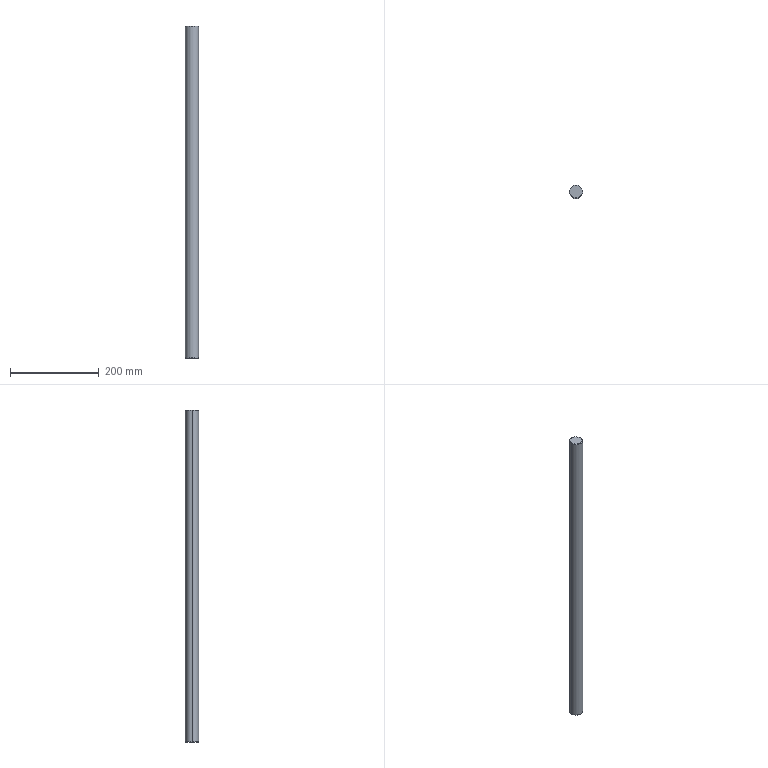Part | STEP file | 2003 Bag feed support shaft | 1 solid | 12 faces | box 30 x 30 x 750 mm | volume 528443 mm3 | cone 6 | cylinder 4 | plane 2 | commonest cylinder face diameters 8.5 x2 30 x2
STEP:
#1=CARTESIAN_POINT('',(0.,0.,0.));
#2=DIRECTION('',(0.,0.,1.));
#3=DIRECTION('',(1.,0.,0.));
#4=AXIS2_PLACEMENT_3D('',#1,#2,#3);
#5=CARTESIAN_POINT('',(-14.,0.,0.));
#6=VERTEX_POINT('',#5);
#7=CARTESIAN_POINT('',(14.,0.,0.));
#8=VERTEX_POINT('',#7);
#9=CARTESIAN_POINT('',(0.,0.,0.));
#10=DIRECTION('',(0.,0.,-1.));
#11=DIRECTION('',(1.,0.,0.));
#12=AXIS2_PLACEMENT_3D('',#9,#10,#11);
#13=CIRCLE('',#12,14.);
#14=CARTESIAN_POINT('',(0.,0.,1.));
#15=DIRECTION('',(0.,0.,1.));
#16=DIRECTION('',(1.,0.,0.));
#17=AXIS2_PLACEMENT_3D('',#14,#15,#16);
#18=CONICAL_SURFACE('',#17,15.,0.7854);
#19=CARTESIAN_POINT('',(6.283,-1.));
#20=DIRECTION('',(-1.,0.));
#21=VECTOR('',#20,1.);
#22=LINE('',#19,#21);
#23=(GEOMETRIC_REPRESENTATION_CONTEXT(2)PARAMETRIC_REPRESENTATION_CONTEXT()REPRESENTATION_CONTEXT('',''));
#24=DEFINITIONAL_REPRESENTATION('',(#22),#23);
#25=PCURVE('',#18,#24);
#26=CARTESIAN_POINT('',(0.,0.,0.));
#27=DIRECTION('',(0.,0.,1.));
#28=DIRECTION('',(1.,0.,0.));
#29=AXIS2_PLACEMENT_3D('',#26,#27,#28);
#30=PLANE('',#29);
#31=CARTESIAN_POINT('',(14.,0.));
#32=CARTESIAN_POINT('',(14.,-24.249));
#33=CARTESIAN_POINT('',(-7.,-12.124));
#34=CARTESIAN_POINT('',(-28.,0.));
#35=CARTESIAN_POINT('',(-7.,12.124));
#36=CARTESIAN_POINT('',(14.,24.249));
#37=CARTESIAN_POINT('',(14.,0.));
#38=(BOUNDED_CURVE()B_SPLINE_CURVE(2,(#31,#32,#33,#34,#35,#36,#37),.UNSPECIFIED.,.T.,.F.)B_SPLINE_CURVE_WITH_KNOTS((1,2,2,2,2,1),(-2.094,0.,2.094,4.189,6.283,8.378),.UNSPECIFIED.)CURVE()GEOMETRIC_REPRESENTATION_ITEM()RATIONAL_B_SPLINE_CURVE((1.,0.5,1.,0.5,1.,0.5,1.))REPRESENTATION_ITEM(''));
#39=(GEOMETRIC_REPRESENTATION_CONTEXT(2)PARAMETRIC_REPRESENTATION_CONTEXT()REPRESENTATION_CONTEXT('',''));
#40=DEFINITIONAL_REPRESENTATION('',(#38),#39);
#41=PCURVE('',#30,#40);
#42=SURFACE_CURVE('',#13,(#25,#41),.PCURVE_S1.);
#43=EDGE_CURVE('',#6,#8,#42,.T.);
#44=ORIENTED_EDGE('',*,*,#43,.F.);
#45=CARTESIAN_POINT('',(-15.,0.,1.));
#46=VERTEX_POINT('',#45);
#47=CARTESIAN_POINT('',(-15.,0.,1.));
#48=DIRECTION('',(-0.7071,0.,0.7071));
#49=VECTOR('',#48,1.);
#50=LINE('',#47,#49);
#51=CARTESIAN_POINT('',(3.142,0.));
#52=DIRECTION('',(0.,1.));
#53=VECTOR('',#52,1.);
#54=LINE('',#51,#53);
#55=(GEOMETRIC_REPRESENTATION_CONTEXT(2)PARAMETRIC_REPRESENTATION_CONTEXT()REPRESENTATION_CONTEXT('',''));
#56=DEFINITIONAL_REPRESENTATION('',(#54),#55);
#57=PCURVE('',#18,#56);
#58=CARTESIAN_POINT('',(0.,0.,1.));
#59=DIRECTION('',(0.,0.,1.));
#60=DIRECTION('',(1.,0.,0.));
#61=AXIS2_PLACEMENT_3D('',#58,#59,#60);
#62=CONICAL_SURFACE('',#61,15.,0.7854);
#63=CARTESIAN_POINT('',(3.142,0.));
#64=DIRECTION('',(0.,1.));
#65=VECTOR('',#64,1.);
#66=LINE('',#63,#65);
#67=(GEOMETRIC_REPRESENTATION_CONTEXT(2)PARAMETRIC_REPRESENTATION_CONTEXT()REPRESENTATION_CONTEXT('',''));
#68=DEFINITIONAL_REPRESENTATION('',(#66),#67);
#69=PCURVE('',#62,#68);
#70=SURFACE_CURVE('',#50,(#57,#69),.PCURVE_S1.);
#71=EDGE_CURVE('',#6,#46,#70,.T.);
#72=ORIENTED_EDGE('',*,*,#71,.T.);
#73=CARTESIAN_POINT('',(15.,0.,1.));
#74=VERTEX_POINT('',#73);
#75=CARTESIAN_POINT('',(0.,0.,1.));
#76=DIRECTION('',(0.,0.,1.));
#77=DIRECTION('',(1.,0.,0.));
#78=AXIS2_PLACEMENT_3D('',#75,#76,#77);
#79=CIRCLE('',#78,15.);
#80=CARTESIAN_POINT('',(0.,0.));
#81=DIRECTION('',(1.,0.));
#82=VECTOR('',#81,1.);
#83=LINE('',#80,#82);
#84=(GEOMETRIC_REPRESENTATION_CONTEXT(2)PARAMETRIC_REPRESENTATION_CONTEXT()REPRESENTATION_CONTEXT('',''));
#85=DEFINITIONAL_REPRESENTATION('',(#83),#84);
#86=PCURVE('',#18,#85);
#87=CARTESIAN_POINT('',(0.,0.,750.));
#88=DIRECTION('',(0.,0.,-1.));
#89=DIRECTION('',(-1.,0.,0.));
#90=AXIS2_PLACEMENT_3D('',#87,#88,#89);
#91=CYLINDRICAL_SURFACE('',#90,15.);
#92=CARTESIAN_POINT('',(3.142,749.));
#93=DIRECTION('',(-1.,0.));
#94=VECTOR('',#93,1.);
#95=LINE('',#92,#94);
#96=(GEOMETRIC_REPRESENTATION_CONTEXT(2)PARAMETRIC_REPRESENTATION_CONTEXT()REPRESENTATION_CONTEXT('',''));
#97=DEFINITIONAL_REPRESENTATION('',(#95),#96);
#98=PCURVE('',#91,#97);
#99=SURFACE_CURVE('',#79,(#86,#98),.PCURVE_S1.);
#100=EDGE_CURVE('',#74,#46,#99,.T.);
#101=ORIENTED_EDGE('',*,*,#100,.F.);
#102=CARTESIAN_POINT('',(15.,0.,1.));
#103=DIRECTION('',(0.7071,0.,0.7071));
#104=VECTOR('',#103,1.);
#105=LINE('',#102,#104);
#106=CARTESIAN_POINT('',(0.,0.));
#107=DIRECTION('',(0.,1.));
#108=VECTOR('',#107,1.);
#109=LINE('',#106,#108);
#110=(GEOMETRIC_REPRESENTATION_CONTEXT(2)PARAMETRIC_REPRESENTATION_CONTEXT()REPRESENTATION_CONTEXT('',''));
#111=DEFINITIONAL_REPRESENTATION('',(#109),#110);
#112=PCURVE('',#18,#111);
#113=CARTESIAN_POINT('',(6.283,0.));
#114=DIRECTION('',(0.,1.));
#115=VECTOR('',#114,1.);
#116=LINE('',#113,#115);
#117=(GEOMETRIC_REPRESENTATION_CONTEXT(2)PARAMETRIC_REPRESENTATION_CONTEXT()REPRESENTATION_CONTEXT('',''));
#118=DEFINITIONAL_REPRESENTATION('',(#116),#117);
#119=PCURVE('',#62,#118);
#120=SURFACE_CURVE('',#105,(#112,#119),.PCURVE_S1.);
#121=EDGE_CURVE('',#8,#74,#120,.T.);
#122=ORIENTED_EDGE('',*,*,#121,.F.);
#123=EDGE_LOOP('',(#44,#72,#101,#122));
#124=FACE_BOUND('',#123,.T.);
#125=ADVANCED_FACE('',(#124),#18,.T.);
#126=CARTESIAN_POINT('',(14.,0.,750.));
#127=VERTEX_POINT('',#126);
#128=CARTESIAN_POINT('',(-14.,0.,750.));
#129=VERTEX_POINT('',#128);
#130=CARTESIAN_POINT('',(0.,0.,750.));
#131=DIRECTION('',(0.,0.,1.));
#132=DIRECTION('',(1.,0.,0.));
#133=AXIS2_PLACEMENT_3D('',#130,#131,#132);
#134=CIRCLE('',#133,14.);
#135=CARTESIAN_POINT('',(0.,0.,750.));
#136=DIRECTION('',(0.,0.,-1.));
#137=DIRECTION('',(-1.,0.,0.));
#138=AXIS2_PLACEMENT_3D('',#135,#136,#137);
#139=CONICAL_SURFACE('',#138,14.,0.7854);
#140=CARTESIAN_POINT('',(3.142,0.));
#141=DIRECTION('',(-1.,0.));
#142=VECTOR('',#141,1.);
#143=LINE('',#140,#142);
#144=(GEOMETRIC_REPRESENTATION_CONTEXT(2)PARAMETRIC_REPRESENTATION_CONTEXT()REPRESENTATION_CONTEXT('',''));
#145=DEFINITIONAL_REPRESENTATION('',(#143),#144);
#146=PCURVE('',#139,#145);
#147=CARTESIAN_POINT('',(0.,0.,750.));
#148=DIRECTION('',(0.,0.,1.));
#149=DIRECTION('',(1.,0.,0.));
#150=AXIS2_PLACEMENT_3D('',#147,#148,#149);
#151=PLANE('',#150);
#152=CARTESIAN_POINT('',(0.,0.));
#153=DIRECTION('',(1.,0.));
#154=AXIS2_PLACEMENT_2D('',#152,#153);
#155=CIRCLE('',#154,14.);
#156=(GEOMETRIC_REPRESENTATION_CONTEXT(2)PARAMETRIC_REPRESENTATION_CONTEXT()REPRESENTATION_CONTEXT('',''));
#157=DEFINITIONAL_REPRESENTATION('',(#155),#156);
#158=PCURVE('',#151,#157);
#159=SURFACE_CURVE('',#134,(#146,#158),.PCURVE_S1.);
#160=EDGE_CURVE('',#127,#129,#159,.T.);
#161=ORIENTED_EDGE('',*,*,#160,.F.);
#162=CARTESIAN_POINT('',(15.,0.,749.));
#163=VERTEX_POINT('',#162);
#164=CARTESIAN_POINT('',(14.,0.,750.));
#165=DIRECTION('',(0.7071,0.,-0.7071));
#166=VECTOR('',#165,1.);
#167=LINE('',#164,#166);
#168=CARTESIAN_POINT('',(3.142,0.));
#169=DIRECTION('',(0.,1.));
#170=VECTOR('',#169,1.);
#171=LINE('',#168,#170);
#172=(GEOMETRIC_REPRESENTATION_CONTEXT(2)PARAMETRIC_REPRESENTATION_CONTEXT()REPRESENTATION_CONTEXT('',''));
#173=DEFINITIONAL_REPRESENTATION('',(#171),#172);
#174=PCURVE('',#139,#173);
#175=CARTESIAN_POINT('',(0.,0.,750.));
#176=DIRECTION('',(0.,0.,-1.));
#177=DIRECTION('',(-1.,0.,0.));
#178=AXIS2_PLACEMENT_3D('',#175,#176,#177);
#179=CONICAL_SURFACE('',#178,14.,0.7854);
#180=CARTESIAN_POINT('',(3.142,0.));
#181=DIRECTION('',(0.,1.));
#182=VECTOR('',#181,1.);
#183=LINE('',#180,#182);
#184=(GEOMETRIC_REPRESENTATION_CONTEXT(2)PARAMETRIC_REPRESENTATION_CONTEXT()REPRESENTATION_CONTEXT('',''));
#185=DEFINITIONAL_REPRESENTATION('',(#183),#184);
#186=PCURVE('',#179,#185);
#187=SURFACE_CURVE('',#167,(#174,#186),.PCURVE_S1.);
#188=EDGE_CURVE('',#127,#163,#187,.T.);
#189=ORIENTED_EDGE('',*,*,#188,.T.);
#190=CARTESIAN_POINT('',(-15.,0.,749.));
#191=VERTEX_POINT('',#190);
#192=CARTESIAN_POINT('',(0.,0.,749.));
#193=DIRECTION('',(0.,0.,-1.));
#194=DIRECTION('',(1.,0.,0.));
#195=AXIS2_PLACEMENT_3D('',#192,#193,#194);
#196=CIRCLE('',#195,15.);
#197=CARTESIAN_POINT('',(-3.142,1.));
#198=DIRECTION('',(1.,0.));
#199=VECTOR('',#198,1.);
#200=LINE('',#197,#199);
#201=(GEOMETRIC_REPRESENTATION_CONTEXT(2)PARAMETRIC_REPRESENTATION_CONTEXT()REPRESENTATION_CONTEXT('',''));
#202=DEFINITIONAL_REPRESENTATION('',(#200),#201);
#203=PCURVE('',#139,#202);
#204=CARTESIAN_POINT('',(-3.142,1.));
#205=DIRECTION('',(1.,0.));
#206=VECTOR('',#205,1.);
#207=LINE('',#204,#206);
#208=(GEOMETRIC_REPRESENTATION_CONTEXT(2)PARAMETRIC_REPRESENTATION_CONTEXT()REPRESENTATION_CONTEXT('',''));
#209=DEFINITIONAL_REPRESENTATION('',(#207),#208);
#210=PCURVE('',#91,#209);
#211=SURFACE_CURVE('',#196,(#203,#210),.PCURVE_S1.);
#212=EDGE_CURVE('',#191,#163,#211,.T.);
#213=ORIENTED_EDGE('',*,*,#212,.F.);
#214=CARTESIAN_POINT('',(-14.,0.,750.));
#215=DIRECTION('',(-0.7071,0.,-0.7071));
#216=VECTOR('',#215,1.);
#217=LINE('',#214,#216);
#218=CARTESIAN_POINT('',(0.,0.));
#219=DIRECTION('',(0.,1.));
#220=VECTOR('',#219,1.);
#221=LINE('',#218,#220);
#222=(GEOMETRIC_REPRESENTATION_CONTEXT(2)PARAMETRIC_REPRESENTATION_CONTEXT()REPRESENTATION_CONTEXT('',''));
#223=DEFINITIONAL_REPRESENTATION('',(#221),#222);
#224=PCURVE('',#139,#223);
#225=CARTESIAN_POINT('',(6.283,0.));
#226=DIRECTION('',(0.,1.));
#227=VECTOR('',#226,1.);
#228=LINE('',#225,#227);
#229=(GEOMETRIC_REPRESENTATION_CONTEXT(2)PARAMETRIC_REPRESENTATION_CONTEXT()REPRESENTATION_CONTEXT('',''));
#230=DEFINITIONAL_REPRESENTATION('',(#228),#229);
#231=PCURVE('',#179,#230);
#232=SURFACE_CURVE('',#217,(#224,#231),.PCURVE_S1.);
#233=EDGE_CURVE('',#129,#191,#232,.T.);
#234=ORIENTED_EDGE('',*,*,#233,.F.);
#235=EDGE_LOOP('',(#161,#189,#213,#234));
#236=FACE_BOUND('',#235,.T.);
#237=ADVANCED_FACE('',(#236),#139,.T.);
#238=CARTESIAN_POINT('',(-4.25,0.,27.5));
#239=VERTEX_POINT('',#238);
#240=CARTESIAN_POINT('',(-4.25,0.,0.));
#241=VERTEX_POINT('',#240);
#242=CARTESIAN_POINT('',(-4.25,0.,0.));
#243=DIRECTION('',(0.,0.,-1.));
#244=VECTOR('',#243,1.);
#245=LINE('',#242,#244);
#246=CARTESIAN_POINT('',(0.,0.,0.));
#247=DIRECTION('',(0.,0.,-1.));
#248=DIRECTION('',(-1.,0.,0.));
#249=AXIS2_PLACEMENT_3D('',#246,#247,#248);
#250=CYLINDRICAL_SURFACE('',#249,4.25);
#251=CARTESIAN_POINT('',(6.283,0.));
#252=DIRECTION('',(0.,1.));
#253=VECTOR('',#252,1.);
#254=LINE('',#251,#253);
#255=(GEOMETRIC_REPRESENTATION_CONTEXT(2)PARAMETRIC_REPRESENTATION_CONTEXT()REPRESENTATION_CONTEXT('',''));
#256=DEFINITIONAL_REPRESENTATION('',(#254),#255);
#257=PCURVE('',#250,#256);
#258=CARTESIAN_POINT('',(0.,0.,0.));
#259=DIRECTION('',(0.,0.,-1.));
#260=DIRECTION('',(-1.,0.,0.));
#261=AXIS2_PLACEMENT_3D('',#258,#259,#260);
#262=CYLINDRICAL_SURFACE('',#261,4.25);
#263=CARTESIAN_POINT('',(0.,0.));
#264=DIRECTION('',(0.,1.));
#265=VECTOR('',#264,1.);
#266=LINE('',#263,#265);
#267=(GEOMETRIC_REPRESENTATION_CONTEXT(2)PARAMETRIC_REPRESENTATION_CONTEXT()REPRESENTATION_CONTEXT('',''));
#268=DEFINITIONAL_REPRESENTATION('',(#266),#267);
#269=PCURVE('',#262,#268);
#270=SURFACE_CURVE('',#245,(#257,#269),.PCURVE_S1.);
#271=EDGE_CURVE('',#239,#241,#270,.T.);
#272=ORIENTED_EDGE('',*,*,#271,.T.);
#273=CARTESIAN_POINT('',(4.25,0.,0.));
#274=VERTEX_POINT('',#273);
#275=CARTESIAN_POINT('',(0.,0.,0.));
#276=DIRECTION('',(0.,0.,-1.));
#277=DIRECTION('',(-1.,0.,0.));
#278=AXIS2_PLACEMENT_3D('',#275,#276,#277);
#279=CIRCLE('',#278,4.25);
#280=CARTESIAN_POINT('',(0.,0.));
#281=DIRECTION('',(1.,0.));
#282=VECTOR('',#281,1.);
#283=LINE('',#280,#282);
#284=(GEOMETRIC_REPRESENTATION_CONTEXT(2)PARAMETRIC_REPRESENTATION_CONTEXT()REPRESENTATION_CONTEXT('',''));
#285=DEFINITIONAL_REPRESENTATION('',(#283),#284);
#286=PCURVE('',#250,#285);
#287=CARTESIAN_POINT('',(-4.25,0.));
#288=CARTESIAN_POINT('',(-4.25,7.361));
#289=CARTESIAN_POINT('',(2.125,3.681));
#290=CARTESIAN_POINT('',(8.5,0.));
#291=CARTESIAN_POINT('',(2.125,-3.681));
#292=CARTESIAN_POINT('',(-4.25,-7.361));
#293=CARTESIAN_POINT('',(-4.25,0.));
#294=(BOUNDED_CURVE()B_SPLINE_CURVE(2,(#287,#288,#289,#290,#291,#292,#293),.UNSPECIFIED.,.T.,.F.)B_SPLINE_CURVE_WITH_KNOTS((1,2,2,2,2,1),(-2.094,0.,2.094,4.189,6.283,8.378),.UNSPECIFIED.)CURVE()GEOMETRIC_REPRESENTATION_ITEM()RATIONAL_B_SPLINE_CURVE((1.,0.5,1.,0.5,1.,0.5,1.))REPRESENTATION_ITEM(''));
#295=(GEOMETRIC_REPRESENTATION_CONTEXT(2)PARAMETRIC_REPRESENTATION_CONTEXT()REPRESENTATION_CONTEXT('',''));
#296=DEFINITIONAL_REPRESENTATION('',(#294),#295);
#297=PCURVE('',#30,#296);
#298=SURFACE_CURVE('',#279,(#286,#297),.PCURVE_S1.);
#299=EDGE_CURVE('',#274,#241,#298,.T.);
#300=ORIENTED_EDGE('',*,*,#299,.F.);
#301=CARTESIAN_POINT('',(4.25,0.,27.5));
#302=VERTEX_POINT('',#301);
#303=CARTESIAN_POINT('',(4.25,0.,0.));
#304=DIRECTION('',(0.,0.,-1.));
#305=VECTOR('',#304,1.);
#306=LINE('',#303,#305);
#307=CARTESIAN_POINT('',(3.142,0.));
#308=DIRECTION('',(0.,1.));
#309=VECTOR('',#308,1.);
#310=LINE('',#307,#309);
#311=(GEOMETRIC_REPRESENTATION_CONTEXT(2)PARAMETRIC_REPRESENTATION_CONTEXT()REPRESENTATION_CONTEXT('',''));
#312=DEFINITIONAL_REPRESENTATION('',(#310),#311);
#313=PCURVE('',#250,#312);
#314=CARTESIAN_POINT('',(3.142,0.));
#315=DIRECTION('',(0.,1.));
#316=VECTOR('',#315,1.);
#317=LINE('',#314,#316);
#318=(GEOMETRIC_REPRESENTATION_CONTEXT(2)PARAMETRIC_REPRESENTATION_CONTEXT()REPRESENTATION_CONTEXT('',''));
#319=DEFINITIONAL_REPRESENTATION('',(#317),#318);
#320=PCURVE('',#262,#319);
#321=SURFACE_CURVE('',#306,(#313,#320),.PCURVE_S1.);
#322=EDGE_CURVE('',#302,#274,#321,.T.);
#323=ORIENTED_EDGE('',*,*,#322,.F.);
#324=CARTESIAN_POINT('',(0.,0.,27.5));
#325=DIRECTION('',(0.,0.,-1.));
#326=DIRECTION('',(-1.,0.,0.));
#327=AXIS2_PLACEMENT_3D('',#324,#325,#326);
#328=CIRCLE('',#327,4.25);
#329=CARTESIAN_POINT('',(0.,-27.5));
#330=DIRECTION('',(1.,0.));
#331=VECTOR('',#330,1.);
#332=LINE('',#329,#331);
#333=(GEOMETRIC_REPRESENTATION_CONTEXT(2)PARAMETRIC_REPRESENTATION_CONTEXT()REPRESENTATION_CONTEXT('',''));
#334=DEFINITIONAL_REPRESENTATION('',(#332),#333);
#335=PCURVE('',#250,#334);
#336=CARTESIAN_POINT('',(0.,0.,27.5));
#337=DIRECTION('',(0.,0.,-1.));
#338=DIRECTION('',(-1.,0.,0.));
#339=AXIS2_PLACEMENT_3D('',#336,#337,#338);
#340=CONICAL_SURFACE('',#339,4.25,1.03);
#341=CARTESIAN_POINT('',(0.,0.));
#342=DIRECTION('',(1.,0.));
#343=VECTOR('',#342,1.);
#344=LINE('',#341,#343);
#345=(GEOMETRIC_REPRESENTATION_CONTEXT(2)PARAMETRIC_REPRESENTATION_CONTEXT()REPRESENTATION_CONTEXT('',''));
#346=DEFINITIONAL_REPRESENTATION('',(#344),#345);
#347=PCURVE('',#340,#346);
#348=SURFACE_CURVE('',#328,(#335,#347),.PCURVE_S1.);
#349=EDGE_CURVE('',#302,#239,#348,.T.);
#350=ORIENTED_EDGE('',*,*,#349,.T.);
#351=EDGE_LOOP('',(#272,#300,#323,#350));
#352=FACE_BOUND('',#351,.F.);
#353=ADVANCED_FACE('',(#352),#250,.F.);
#354=ORIENTED_EDGE('',*,*,#349,.F.);
#355=CARTESIAN_POINT('',(0.,0.,30.054));
#356=VERTEX_POINT('',#355);
#357=CARTESIAN_POINT('',(4.25,0.,27.5));
#358=DIRECTION('',(0.8572,0.,-0.515));
#359=VECTOR('',#358,1.);
#360=LINE('',#357,#359);
#361=CARTESIAN_POINT('',(3.142,0.));
#362=DIRECTION('',(0.,1.));
#363=VECTOR('',#362,1.);
#364=LINE('',#361,#363);
#365=(GEOMETRIC_REPRESENTATION_CONTEXT(2)PARAMETRIC_REPRESENTATION_CONTEXT()REPRESENTATION_CONTEXT('',''));
#366=DEFINITIONAL_REPRESENTATION('',(#364),#365);
#367=PCURVE('',#340,#366);
#368=CARTESIAN_POINT('',(0.,0.,27.5));
#369=DIRECTION('',(0.,0.,-1.));
#370=DIRECTION('',(-1.,0.,0.));
#371=AXIS2_PLACEMENT_3D('',#368,#369,#370);
#372=CONICAL_SURFACE('',#371,4.25,1.03);
#373=CARTESIAN_POINT('',(3.142,0.));
#374=DIRECTION('',(0.,1.));
#375=VECTOR('',#374,1.);
#376=LINE('',#373,#375);
#377=(GEOMETRIC_REPRESENTATION_CONTEXT(2)PARAMETRIC_REPRESENTATION_CONTEXT()REPRESENTATION_CONTEXT('',''));
#378=DEFINITIONAL_REPRESENTATION('',(#376),#377);
#379=PCURVE('',#372,#378);
#380=SURFACE_CURVE('',#360,(#367,#379),.PCURVE_S1.);
#381=EDGE_CURVE('',#356,#302,#380,.T.);
#382=ORIENTED_EDGE('',*,*,#381,.F.);
#383=CARTESIAN_POINT('',(-4.25,0.,27.5));
#384=DIRECTION('',(-0.8572,0.,-0.515));
#385=VECTOR('',#384,1.);
#386=LINE('',#383,#385);
#387=CARTESIAN_POINT('',(6.283,0.));
#388=DIRECTION('',(0.,1.));
#389=VECTOR('',#388,1.);
#390=LINE('',#387,#389);
#391=(GEOMETRIC_REPRESENTATION_CONTEXT(2)PARAMETRIC_REPRESENTATION_CONTEXT()REPRESENTATION_CONTEXT('',''));
#392=DEFINITIONAL_REPRESENTATION('',(#390),#391);
#393=PCURVE('',#340,#392);
#394=CARTESIAN_POINT('',(0.,0.));
#395=DIRECTION('',(0.,1.));
#396=VECTOR('',#395,1.);
#397=LINE('',#394,#396);
#398=(GEOMETRIC_REPRESENTATION_CONTEXT(2)PARAMETRIC_REPRESENTATION_CONTEXT()REPRESENTATION_CONTEXT('',''));
#399=DEFINITIONAL_REPRESENTATION('',(#397),#398);
#400=PCURVE('',#372,#399);
#401=SURFACE_CURVE('',#386,(#393,#400),.PCURVE_S1.);
#402=EDGE_CURVE('',#356,#239,#401,.T.);
#403=ORIENTED_EDGE('',*,*,#402,.T.);
#404=EDGE_LOOP('',(#354,#382,#403));
#405=FACE_BOUND('',#404,.F.);
#406=ADVANCED_FACE('',(#405),#340,.F.);
#407=ORIENTED_EDGE('',*,*,#212,.T.);
#408=CARTESIAN_POINT('',(15.,0.,750.));
#409=DIRECTION('',(0.,0.,-1.));
#410=VECTOR('',#409,1.);
#411=LINE('',#408,#410);
#412=CARTESIAN_POINT('',(3.142,0.));
#413=DIRECTION('',(0.,1.));
#414=VECTOR('',#413,1.);
#415=LINE('',#412,#414);
#416=(GEOMETRIC_REPRESENTATION_CONTEXT(2)PARAMETRIC_REPRESENTATION_CONTEXT()REPRESENTATION_CONTEXT('',''));
#417=DEFINITIONAL_REPRESENTATION('',(#415),#416);
#418=PCURVE('',#91,#417);
#419=CARTESIAN_POINT('',(0.,0.,750.));
#420=DIRECTION('',(0.,0.,-1.));
#421=DIRECTION('',(-1.,0.,0.));
#422=AXIS2_PLACEMENT_3D('',#419,#420,#421);
#423=CYLINDRICAL_SURFACE('',#422,15.);
#424=CARTESIAN_POINT('',(3.142,0.));
#425=DIRECTION('',(0.,1.));
#426=VECTOR('',#425,1.);
#427=LINE('',#424,#426);
#428=(GEOMETRIC_REPRESENTATION_CONTEXT(2)PARAMETRIC_REPRESENTATION_CONTEXT()REPRESENTATION_CONTEXT('',''));
#429=DEFINITIONAL_REPRESENTATION('',(#427),#428);
#430=PCURVE('',#423,#429);
#431=SURFACE_CURVE('',#411,(#418,#430),.PCURVE_S1.);
#432=EDGE_CURVE('',#163,#74,#431,.T.);
#433=ORIENTED_EDGE('',*,*,#432,.T.);
#434=ORIENTED_EDGE('',*,*,#100,.T.);
#435=CARTESIAN_POINT('',(-15.,0.,750.));
#436=DIRECTION('',(0.,0.,-1.));
#437=VECTOR('',#436,1.);
#438=LINE('',#435,#437);
#439=CARTESIAN_POINT('',(0.,0.));
#440=DIRECTION('',(0.,1.));
#441=VECTOR('',#440,1.);
#442=LINE('',#439,#441);
#443=(GEOMETRIC_REPRESENTATION_CONTEXT(2)PARAMETRIC_REPRESENTATION_CONTEXT()REPRESENTATION_CONTEXT('',''));
#444=DEFINITIONAL_REPRESENTATION('',(#442),#443);
#445=PCURVE('',#91,#444);
#446=CARTESIAN_POINT('',(6.283,0.));
#447=DIRECTION('',(0.,1.));
#448=VECTOR('',#447,1.);
#449=LINE('',#446,#448);
#450=(GEOMETRIC_REPRESENTATION_CONTEXT(2)PARAMETRIC_REPRESENTATION_CONTEXT()REPRESENTATION_CONTEXT('',''));
#451=DEFINITIONAL_REPRESENTATION('',(#449),#450);
#452=PCURVE('',#423,#451);
#453=SURFACE_CURVE('',#438,(#445,#452),.PCURVE_S1.);
#454=EDGE_CURVE('',#191,#46,#453,.T.);
#455=ORIENTED_EDGE('',*,*,#454,.F.);
#456=EDGE_LOOP('',(#407,#433,#434,#455));
#457=FACE_BOUND('',#456,.T.);
#458=ADVANCED_FACE('',(#457),#91,.T.);
#459=ORIENTED_EDGE('',*,*,#432,.F.);
#460=CARTESIAN_POINT('',(0.,0.,749.));
#461=DIRECTION('',(0.,0.,-1.));
#462=DIRECTION('',(1.,0.,0.));
#463=AXIS2_PLACEMENT_3D('',#460,#461,#462);
#464=CIRCLE('',#463,15.);
#465=CARTESIAN_POINT('',(3.142,1.));
#466=DIRECTION('',(1.,0.));
#467=VECTOR('',#466,1.);
#468=LINE('',#465,#467);
#469=(GEOMETRIC_REPRESENTATION_CONTEXT(2)PARAMETRIC_REPRESENTATION_CONTEXT()REPRESENTATION_CONTEXT('',''));
#470=DEFINITIONAL_REPRESENTATION('',(#468),#469);
#471=PCURVE('',#423,#470);
#472=CARTESIAN_POINT('',(3.142,1.));
#473=DIRECTION('',(1.,0.));
#474=VECTOR('',#473,1.);
#475=LINE('',#472,#474);
#476=(GEOMETRIC_REPRESENTATION_CONTEXT(2)PARAMETRIC_REPRESENTATION_CONTEXT()REPRESENTATION_CONTEXT('',''));
#477=DEFINITIONAL_REPRESENTATION('',(#475),#476);
#478=PCURVE('',#179,#477);
#479=SURFACE_CURVE('',#464,(#471,#478),.PCURVE_S1.);
#480=EDGE_CURVE('',#163,#191,#479,.T.);
#481=ORIENTED_EDGE('',*,*,#480,.T.);
#482=ORIENTED_EDGE('',*,*,#454,.T.);
#483=CARTESIAN_POINT('',(0.,0.,1.));
#484=DIRECTION('',(0.,0.,1.));
#485=DIRECTION('',(1.,0.,0.));
#486=AXIS2_PLACEMENT_3D('',#483,#484,#485);
#487=CIRCLE('',#486,15.);
#488=CARTESIAN_POINT('',(9.425,749.));
#489=DIRECTION('',(-1.,0.));
#490=VECTOR('',#489,1.);
#491=LINE('',#488,#490);
#492=(GEOMETRIC_REPRESENTATION_CONTEXT(2)PARAMETRIC_REPRESENTATION_CONTEXT()REPRESENTATION_CONTEXT('',''));
#493=DEFINITIONAL_REPRESENTATION('',(#491),#492);
#494=PCURVE('',#423,#493);
#495=CARTESIAN_POINT('',(0.,0.));
#496=DIRECTION('',(1.,0.));
#497=VECTOR('',#496,1.);
#498=LINE('',#495,#497);
#499=(GEOMETRIC_REPRESENTATION_CONTEXT(2)PARAMETRIC_REPRESENTATION_CONTEXT()REPRESENTATION_CONTEXT('',''));
#500=DEFINITIONAL_REPRESENTATION('',(#498),#499);
#501=PCURVE('',#62,#500);
#502=SURFACE_CURVE('',#487,(#494,#501),.PCURVE_S1.);
#503=EDGE_CURVE('',#46,#74,#502,.T.);
#504=ORIENTED_EDGE('',*,*,#503,.T.);
#505=EDGE_LOOP('',(#459,#481,#482,#504));
#506=FACE_BOUND('',#505,.T.);
#507=ADVANCED_FACE('',(#506),#423,.T.);
#508=CARTESIAN_POINT('',(0.,0.,750.));
#509=DIRECTION('',(0.,0.,1.));
#510=DIRECTION('',(1.,0.,0.));
#511=AXIS2_PLACEMENT_3D('',#508,#509,#510);
#512=CIRCLE('',#511,14.);
#513=CARTESIAN_POINT('',(0.,0.));
#514=DIRECTION('',(1.,0.));
#515=AXIS2_PLACEMENT_2D('',#513,#514);
#516=CIRCLE('',#515,14.);
#517=(GEOMETRIC_REPRESENTATION_CONTEXT(2)PARAMETRIC_REPRESENTATION_CONTEXT()REPRESENTATION_CONTEXT('',''));
#518=DEFINITIONAL_REPRESENTATION('',(#516),#517);
#519=PCURVE('',#151,#518);
#520=CARTESIAN_POINT('',(9.425,0.));
#521=DIRECTION('',(-1.,0.));
#522=VECTOR('',#521,1.);
#523=LINE('',#520,#522);
#524=(GEOMETRIC_REPRESENTATION_CONTEXT(2)PARAMETRIC_REPRESENTATION_CONTEXT()REPRESENTATION_CONTEXT('',''));
#525=DEFINITIONAL_REPRESENTATION('',(#523),#524);
#526=PCURVE('',#179,#525);
#527=SURFACE_CURVE('',#512,(#519,#526),.PCURVE_S1.);
#528=EDGE_CURVE('',#129,#127,#527,.T.);
#529=ORIENTED_EDGE('',*,*,#528,.T.);
#530=ORIENTED_EDGE('',*,*,#160,.T.);
#531=EDGE_LOOP('',(#529,#530));
#532=FACE_BOUND('',#531,.T.);
#533=ADVANCED_FACE('',(#532),#151,.T.);
#534=CARTESIAN_POINT('',(0.,0.,0.));
#535=DIRECTION('',(0.,0.,-1.));
#536=DIRECTION('',(1.,0.,0.));
#537=AXIS2_PLACEMENT_3D('',#534,#535,#536);
#538=CIRCLE('',#537,14.);
#539=CARTESIAN_POINT('',(14.,0.));
#540=CARTESIAN_POINT('',(14.,-24.249));
#541=CARTESIAN_POINT('',(-7.,-12.124));
#542=CARTESIAN_POINT('',(-28.,0.));
#543=CARTESIAN_POINT('',(-7.,12.124));
#544=CARTESIAN_POINT('',(14.,24.249));
#545=CARTESIAN_POINT('',(14.,0.));
#546=(BOUNDED_CURVE()B_SPLINE_CURVE(2,(#539,#540,#541,#542,#543,#544,#545),.UNSPECIFIED.,.T.,.F.)B_SPLINE_CURVE_WITH_KNOTS((1,2,2,2,2,1),(-2.094,0.,2.094,4.189,6.283,8.378),.UNSPECIFIED.)CURVE()GEOMETRIC_REPRESENTATION_ITEM()RATIONAL_B_SPLINE_CURVE((1.,0.5,1.,0.5,1.,0.5,1.))REPRESENTATION_ITEM(''));
#547=(GEOMETRIC_REPRESENTATION_CONTEXT(2)PARAMETRIC_REPRESENTATION_CONTEXT()REPRESENTATION_CONTEXT('',''));
#548=DEFINITIONAL_REPRESENTATION('',(#546),#547);
#549=PCURVE('',#30,#548);
#550=CARTESIAN_POINT('',(6.283,-1.));
#551=DIRECTION('',(-1.,0.));
#552=VECTOR('',#551,1.);
#553=LINE('',#550,#552);
#554=(GEOMETRIC_REPRESENTATION_CONTEXT(2)PARAMETRIC_REPRESENTATION_CONTEXT()REPRESENTATION_CONTEXT('',''));
#555=DEFINITIONAL_REPRESENTATION('',(#553),#554);
#556=PCURVE('',#62,#555);
#557=SURFACE_CURVE('',#538,(#549,#556),.PCURVE_S1.);
#558=EDGE_CURVE('',#8,#6,#557,.T.);
#559=ORIENTED_EDGE('',*,*,#558,.T.);
#560=ORIENTED_EDGE('',*,*,#43,.T.);
#561=EDGE_LOOP('',(#559,#560));
#562=FACE_BOUND('',#561,.T.);
#563=CARTESIAN_POINT('',(0.,0.,0.));
#564=DIRECTION('',(0.,0.,-1.));
#565=DIRECTION('',(-1.,0.,0.));
#566=AXIS2_PLACEMENT_3D('',#563,#564,#565);
#567=CIRCLE('',#566,4.25);
#568=CARTESIAN_POINT('',(-4.25,0.));
#569=CARTESIAN_POINT('',(-4.25,7.361));
#570=CARTESIAN_POINT('',(2.125,3.681));
#571=CARTESIAN_POINT('',(8.5,0.));
#572=CARTESIAN_POINT('',(2.125,-3.681));
#573=CARTESIAN_POINT('',(-4.25,-7.361));
#574=CARTESIAN_POINT('',(-4.25,0.));
#575=(BOUNDED_CURVE()B_SPLINE_CURVE(2,(#568,#569,#570,#571,#572,#573,#574),.UNSPECIFIED.,.T.,.F.)B_SPLINE_CURVE_WITH_KNOTS((1,2,2,2,2,1),(-2.094,0.,2.094,4.189,6.283,8.378),.UNSPECIFIED.)CURVE()GEOMETRIC_REPRESENTATION_ITEM()RATIONAL_B_SPLINE_CURVE((1.,0.5,1.,0.5,1.,0.5,1.))REPRESENTATION_ITEM(''));
#576=(GEOMETRIC_REPRESENTATION_CONTEXT(2)PARAMETRIC_REPRESENTATION_CONTEXT()REPRESENTATION_CONTEXT('',''));
#577=DEFINITIONAL_REPRESENTATION('',(#575),#576);
#578=PCURVE('',#30,#577);
#579=CARTESIAN_POINT('',(0.,0.));
#580=DIRECTION('',(1.,0.));
#581=VECTOR('',#580,1.);
#582=LINE('',#579,#581);
#583=(GEOMETRIC_REPRESENTATION_CONTEXT(2)PARAMETRIC_REPRESENTATION_CONTEXT()REPRESENTATION_CONTEXT('',''));
#584=DEFINITIONAL_REPRESENTATION('',(#582),#583);
#585=PCURVE('',#262,#584);
#586=SURFACE_CURVE('',#567,(#578,#585),.PCURVE_S1.);
#587=EDGE_CURVE('',#241,#274,#586,.T.);
#588=ORIENTED_EDGE('',*,*,#587,.F.);
#589=ORIENTED_EDGE('',*,*,#299,.F.);
#590=EDGE_LOOP('',(#588,#589));
#591=FACE_BOUND('',#590,.T.);
#592=ADVANCED_FACE('',(#562,#591),#30,.F.);
#593=CARTESIAN_POINT('',(0.,0.,27.5));
#594=DIRECTION('',(0.,0.,-1.));
#595=DIRECTION('',(-1.,0.,0.));
#596=AXIS2_PLACEMENT_3D('',#593,#594,#595);
#597=CIRCLE('',#596,4.25);
#598=CARTESIAN_POINT('',(0.,0.));
#599=DIRECTION('',(1.,0.));
#600=VECTOR('',#599,1.);
#601=LINE('',#598,#600);
#602=(GEOMETRIC_REPRESENTATION_CONTEXT(2)PARAMETRIC_REPRESENTATION_CONTEXT()REPRESENTATION_CONTEXT('',''));
#603=DEFINITIONAL_REPRESENTATION('',(#601),#602);
#604=PCURVE('',#372,#603);
#605=CARTESIAN_POINT('',(0.,-27.5));
#606=DIRECTION('',(1.,0.));
#607=VECTOR('',#606,1.);
#608=LINE('',#605,#607);
#609=(GEOMETRIC_REPRESENTATION_CONTEXT(2)PARAMETRIC_REPRESENTATION_CONTEXT()REPRESENTATION_CONTEXT('',''));
#610=DEFINITIONAL_REPRESENTATION('',(#608),#609);
#611=PCURVE('',#262,#610);
#612=SURFACE_CURVE('',#597,(#604,#611),.PCURVE_S1.);
#613=EDGE_CURVE('',#239,#302,#612,.T.);
#614=ORIENTED_EDGE('',*,*,#613,.F.);
#615=ORIENTED_EDGE('',*,*,#402,.F.);
#616=ORIENTED_EDGE('',*,*,#381,.T.);
#617=EDGE_LOOP('',(#614,#615,#616));
#618=FACE_BOUND('',#617,.F.);
#619=ADVANCED_FACE('',(#618),#372,.F.);
#620=ORIENTED_EDGE('',*,*,#587,.F.);
#621=ORIENTED_EDGE('',*,*,#271,.F.);
#622=ORIENTED_EDGE('',*,*,#613,.T.);
#623=ORIENTED_EDGE('',*,*,#322,.T.);
#624=EDGE_LOOP('',(#620,#621,#622,#623));
#625=FACE_BOUND('',#624,.F.);
#626=ADVANCED_FACE('',(#625),#262,.F.);
#627=ORIENTED_EDGE('',*,*,#188,.F.);
#628=ORIENTED_EDGE('',*,*,#528,.F.);
#629=ORIENTED_EDGE('',*,*,#233,.T.);
#630=ORIENTED_EDGE('',*,*,#480,.F.);
#631=EDGE_LOOP('',(#627,#628,#629,#630));
#632=FACE_BOUND('',#631,.T.);
#633=ADVANCED_FACE('',(#632),#179,.T.);
#634=ORIENTED_EDGE('',*,*,#71,.F.);
#635=ORIENTED_EDGE('',*,*,#558,.F.);
#636=ORIENTED_EDGE('',*,*,#121,.T.);
#637=ORIENTED_EDGE('',*,*,#503,.F.);
#638=EDGE_LOOP('',(#634,#635,#636,#637));
#639=FACE_BOUND('',#638,.T.);
#640=ADVANCED_FACE('',(#639),#62,.T.);
#641=CLOSED_SHELL('',(#125,#237,#353,#406,#458,#507,#533,#592,#619,#626,#633,#640));
#642=MANIFOLD_SOLID_BREP('',#641);
#643=(LENGTH_UNIT()NAMED_UNIT(*)SI_UNIT(.MILLI.,.METRE.));
#644=UNCERTAINTY_MEASURE_WITH_UNIT(LENGTH_MEASURE(0.0000001),#643,'','');
#645=(NAMED_UNIT(*)PLANE_ANGLE_UNIT()SI_UNIT($,.RADIAN.));
#646=(NAMED_UNIT(*)SI_UNIT($,.STERADIAN.)SOLID_ANGLE_UNIT());
#647=(GEOMETRIC_REPRESENTATION_CONTEXT(3)GLOBAL_UNCERTAINTY_ASSIGNED_CONTEXT((#644))GLOBAL_UNIT_ASSIGNED_CONTEXT((#643,#645,#646))REPRESENTATION_CONTEXT('',''));
#648=ADVANCED_BREP_SHAPE_REPRESENTATION('',(#4,#642),#647);